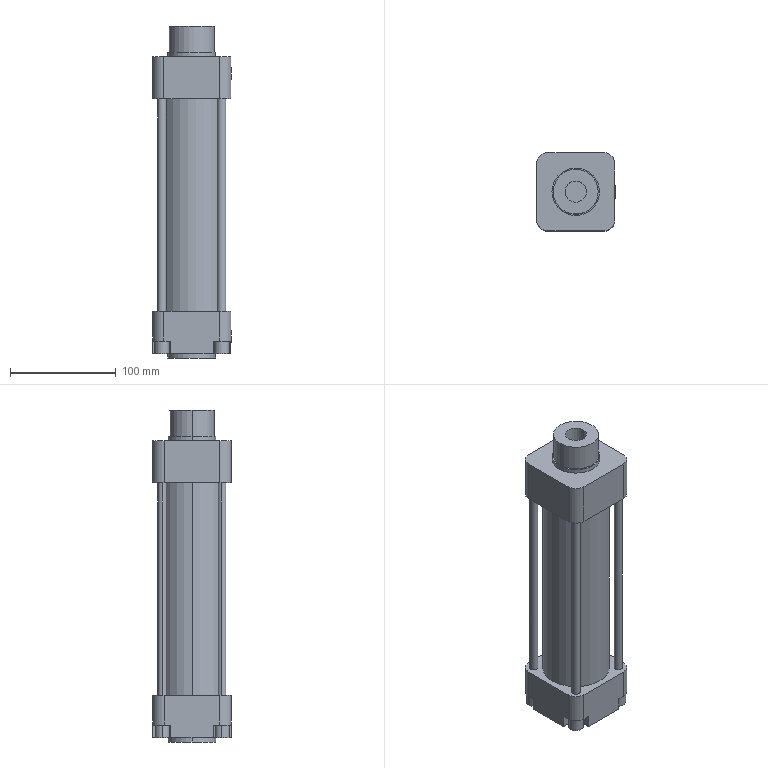Part | NX | 19 solids | 177 faces | box 74.5 x 74 x 314 mm | volume 475496 mm3 | plane 99 | cylinder 74 | cone 4 | commonest cylinder face diameters 10 x12 8 x8 14 x8 21.378 x8 7.215 x4 7.511 x4